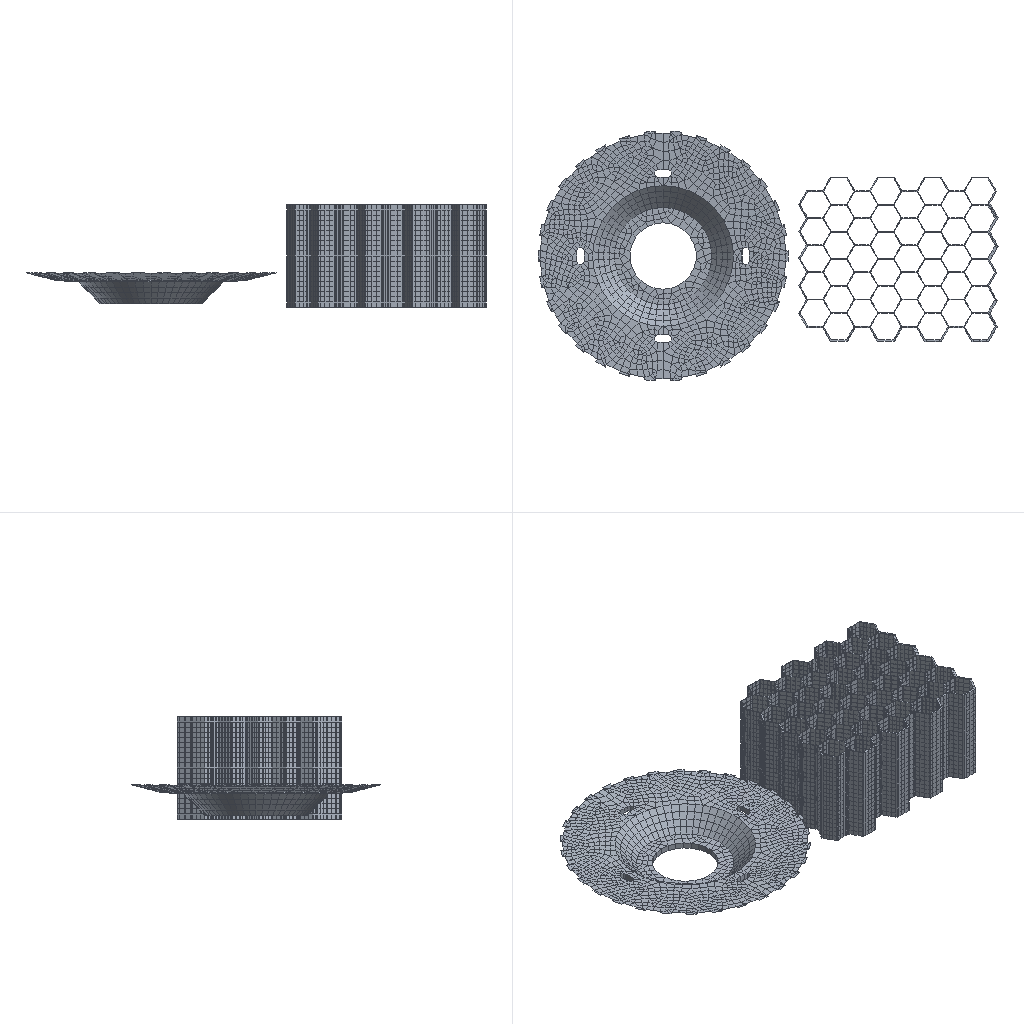Simulation study | abaqus
Set-up summary:
category,name,step,type,value,unit,region
solver,abaqus
solver,version,,,Abaqus/Explicit 2020
units,not stated in the deck,,not stated
analysis,deck,,dynamic temperature-displacement,dynamic temperature-displacement
load_step,Step-1,Step-1,dynamic temperature-displacement,nlgeom=True
contact,interactions,,,general=1 pairs=0 ties=0
load_step,requested,,,1
mesh,nodes,,,29105
mesh,elements,,,17374
element_type,S3,,shell,570
element_type,S4R,,shell,2724
element_type,C3D8RT,,solid,14080
load,load commands in deck,,count,3
bc,support commands in deck,,count,7
material,MATERIAL-1,,in results
material,STEL,,in results
check,setup vs results,,match,"per instance, exact: element labels, types and connectivity; labels of the nodes the elements use; coordinates of those nodes at SINGLE_PRECISION in 1 of 2 instance(s)"
Abaqus input file, long lists of numbers shortened:
*Heading
** Job name: Job-1 Model name: Model-1
** Generated by: Abaqus/CAE 2020
*Preprint, echo=NO, model=NO, history=NO, contact=NO
**
** PARTS
**
*Part, name=daoju
*Node
      1,           0.,   11.898,         -6.5
      2,           0.,   11.898,          6.5
** (2999 more lines like these left out)
*Element, type=S4R
 1,   1, 325, 348,   4
 2, 325, 326, 347, 348
** (2722 more lines like these left out)
*Element, type=S3
571,  392,  190,  185
572, 1557, 1549, 1525
** (568 more lines like these left out)
*Node
   3002, 3.9801022e-16,   10.698,           0.
*Nset, nset=daoju-RefPt_, internal
3002,
*Nset, nset=Set-4, generate
    1,  3001,     1
*Elset, elset=Set-4, generate
    1,  3294,     1
** Section: tol
*Shell Section, elset=Set-4, material=stel
2., 5
*End Part
**
*Part, name=fengwoxin
*Node
      1,  -17.1,   10.086,           0.
      2,  -17.186,   10.036,           0.
** (26101 more lines like these left out)
*Element, type=C3D8RT
    1,   576,   573,     2,     1,  1819,  1816,  1245,  1244
    2,   575,   574,   573,   576,  1818,  1817,  1816,  1819
** (14078 more lines like these left out)
*Nset, nset=Set-2, generate
     1,  26103,      1
*Elset, elset=Set-2, generate
     1,  14080,      1
** Section: Section-1
*Solid Section, elset=Set-2, material=Material-1
,
*End Part
**
**
** ASSEMBLY
**
*Assembly, name=Assembly
**
*Instance, name=fengwoxin-1, part=fengwoxin
*End Instance
**
*Instance, name=daoju-1, part=daoju
        -50.,           0.,         -10.
        -50.,           0.,         -10., -49.,           0.,         -10., 90.
*End Instance
**
*Nset, nset=Set-1, instance=fengwoxin-1, generate
    1,  1243,     1
*Elset, elset=Set-1, instance=fengwoxin-1, generate
   1,  704,    1
*Nset, nset=Set-2, instance=daoju-1
 3002,
*Nset, nset=Set-5, instance=daoju-1
 3002,
*Nset, nset=b_Set-3, instance=daoju-1, generate
    1,  3001,     1
*Elset, elset=b_Set-3, instance=daoju-1, generate
    1,  3294,     1
*Nset, nset=_PickedSet11, internal, instance=daoju-1
 3002,
** Constraint: Constraint-1
*Rigid Body, ref node=_PickedSet11, elset=b_Set-3
*End Assembly
**
** MATERIALS
**
*Material, name=Material-1
*Conductivity
20.,
*Damage Initiation, criterion=SHEAR
 0.0001,0.,0.
*Damage Evolution, type=DISPLACEMENT
 1e-05,
*Density
 1.33e-09,
*Elastic
2010., 0.25
*Expansion
 1e-06,
*Plastic
400.,0.
*Specific Heat
 8e+08,
*Material, name=stel
*Conductivity
46.,
*Density
 7.8e-09,
*Elastic
210000., 0.3
*Expansion
 1e-06,
*Specific Heat
 4.6e+08,
**
** INTERACTION PROPERTIES
**
*Surface Interaction, name=IntProp-1
*Friction
 0.2,
*Surface Behavior, pressure-overclosure=HARD
*Gap Conductance
 0.5,    0.
  0., 0.001
** ----------------------------------------------------------------
**
** STEP: Step-1
**
*Step, name=Step-1, nlgeom=YES
*Dynamic Temperature-displacement, Explicit
, 0.1
*Bulk Viscosity
0.06, 1.2
** Mass Scaling: Semi-Automatic
**               Whole Model
*Fixed Mass Scaling, factor=5000.
**
** BOUNDARY CONDITIONS
**
** Name: BC-1 Type: 对称/反对称/完全固定
*Boundary
Set-1, ENCASTRE
** Name: BC-2 Type: 速度/角速度
*Boundary, type=VELOCITY
Set-5, 1, 1, 450.
Set-5, 2, 2
Set-5, 3, 3, 150.
Set-5, 4, 4
Set-5, 5, 5
Set-5, 6, 6, 62.8
**
** INTERACTIONS
**
** Interaction: Int-1
*Contact, op=NEW
*Contact Inclusions, ALL EXTERIOR
*Contact Property Assignment
 ,  , IntProp-1
**
** OUTPUT REQUESTS
**
*Restart, write, number interval=1, time marks=NO
**
** FIELD OUTPUT: F-Output-1
**
*Output, field, number interval=50
*Node Output
A, CF, NT, RF, RM, RT, U, V
*Element Output, directions=YES
E, EVF, HFL, LE, MISES, MISESMAX, MISESONLY, PE, PEEQ, PEEQMAX, PEEQT, PEEQVAVG, PEVAVG, S, SF, SSAVG
STATUS, SVAVG, TEMP, YIELDPOT
*Contact Output
CDISP, CSTRESS
**
** HISTORY OUTPUT: H-Output-1
**
*Output, history, time interval=5e-06
*Node Output, nset=Set-5
RF1, RF2, RF3
*End Step
Results summary:
result,step,Step-1,completed,increments=48149 time=0.1/0.1
result,analysis,,,"dynamic temperature-displacement, explict"
result,last_loadstep,,,1
result,analysis steps,,count,1
result,primary field,,,"U, UR, NT11"
result,reaction total,,FX,122.57,model units
result,reaction total,,FY,-61.553,model units
result,reaction total,,FZ,-40.422,model units